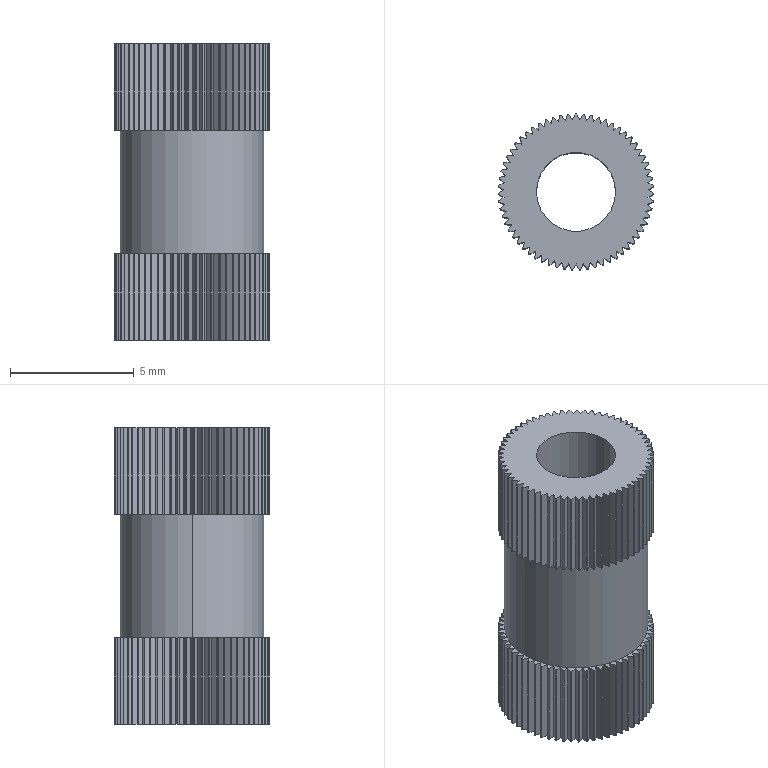Part | SolidWorks | features ICE 2, CirPattern 1, Extrusion 1 | 1 solid | 386 faces | box 6.299 x 6.297 x 12 mm | volume 240.496 mm3 | plane 256 | cylinder 130 | commonest cylinder face diameters 6.3 x126 3.2 x2 5.8 x2